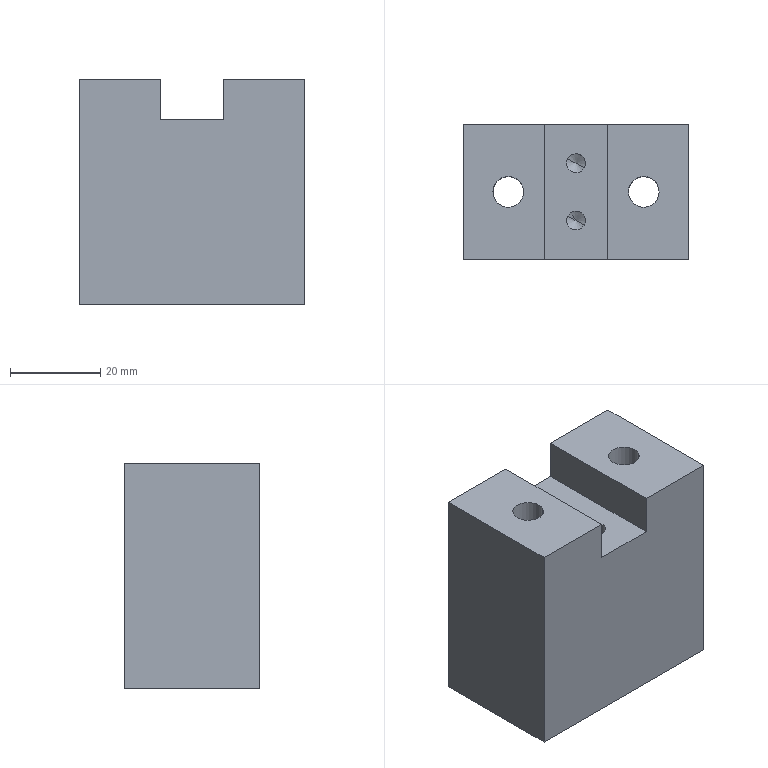Part | STEP file | 20307 | 1 solid | 26 faces | box 50 x 30 x 50 mm | volume 67161 mm3 | cylinder 12 | plane 10 | cone 4 | commonest cylinder face diameters 6.8 x8 4.2 x4
STEP:
#1=CARTESIAN_POINT('',(-17.984,-1.63,0.));
#2=VERTEX_POINT('',#1);
#3=CARTESIAN_POINT('',(-12.016,1.63,0.));
#4=VERTEX_POINT('',#3);
#5=CARTESIAN_POINT('',(-15.,0.,0.));
#6=DIRECTION('',(0.,0.,1.));
#7=AXIS2_PLACEMENT_3D('',#5,#6,$);
#8=CIRCLE('',#7,3.4);
#9=EDGE_CURVE('',#2,#4,#8,.T.);
#10=ORIENTED_EDGE('',*,*,#9,.F.);
#11=CARTESIAN_POINT('',(-17.984,-1.63,15.));
#12=VERTEX_POINT('',#11);
#13=CARTESIAN_POINT('',(-17.984,-1.63,7.345));
#14=DIRECTION('',(0.,0.,1.));
#15=VECTOR('',#14,1.);
#16=LINE('',#13,#15);
#17=EDGE_CURVE('',#12,#2,#16,.F.);
#18=ORIENTED_EDGE('',*,*,#17,.F.);
#19=CARTESIAN_POINT('',(-12.016,-1.63,15.));
#20=VERTEX_POINT('',#19);
#21=CARTESIAN_POINT('',(-15.,0.,15.));
#22=DIRECTION('',(0.,0.,1.));
#23=AXIS2_PLACEMENT_3D('',#21,#22,$);
#24=CIRCLE('',#23,3.4);
#25=EDGE_CURVE('',#20,#12,#24,.F.);
#26=ORIENTED_EDGE('',*,*,#25,.F.);
#27=CARTESIAN_POINT('',(-12.016,1.63,15.));
#28=VERTEX_POINT('',#27);
#29=CARTESIAN_POINT('',(-15.,0.,15.));
#30=DIRECTION('',(0.,0.,1.));
#31=AXIS2_PLACEMENT_3D('',#29,#30,$);
#32=CIRCLE('',#31,3.4);
#33=EDGE_CURVE('',#28,#20,#32,.F.);
#34=ORIENTED_EDGE('',*,*,#33,.F.);
#35=CARTESIAN_POINT('',(-12.016,1.63,7.345));
#36=DIRECTION('',(0.,0.,1.));
#37=VECTOR('',#36,1.);
#38=LINE('',#35,#37);
#39=EDGE_CURVE('',#28,#4,#38,.F.);
#40=ORIENTED_EDGE('',*,*,#39,.T.);
#41=EDGE_LOOP('',(#10,#18,#26,#34,#40));
#42=FACE_OUTER_BOUND('',#41,.T.);
#43=CARTESIAN_POINT('',(-15.,0.,0.1));
#44=DIRECTION('',(0.,0.,1.));
#45=DIRECTION('',(0.8776,0.4794,0.));
#46=AXIS2_PLACEMENT_3D('',#43,#44,#45);
#47=CYLINDRICAL_SURFACE('',#46,3.4);
#48=ADVANCED_FACE('',(#42),#47,.F.);
#49=CARTESIAN_POINT('',(-15.,0.,0.));
#50=DIRECTION('',(0.,0.,1.));
#51=AXIS2_PLACEMENT_3D('',#49,#50,$);
#52=CIRCLE('',#51,3.4);
#53=EDGE_CURVE('',#4,#2,#52,.T.);
#54=ORIENTED_EDGE('',*,*,#53,.F.);
#55=ORIENTED_EDGE('',*,*,#39,.F.);
#56=CARTESIAN_POINT('',(-17.984,1.63,15.));
#57=VERTEX_POINT('',#56);
#58=CARTESIAN_POINT('',(-15.,0.,15.));
#59=DIRECTION('',(0.,0.,1.));
#60=AXIS2_PLACEMENT_3D('',#58,#59,$);
#61=CIRCLE('',#60,3.4);
#62=EDGE_CURVE('',#57,#28,#61,.F.);
#63=ORIENTED_EDGE('',*,*,#62,.F.);
#64=CARTESIAN_POINT('',(-15.,0.,15.));
#65=DIRECTION('',(0.,0.,1.));
#66=AXIS2_PLACEMENT_3D('',#64,#65,$);
#67=CIRCLE('',#66,3.4);
#68=EDGE_CURVE('',#12,#57,#67,.F.);
#69=ORIENTED_EDGE('',*,*,#68,.F.);
#70=ORIENTED_EDGE('',*,*,#17,.T.);
#71=EDGE_LOOP('',(#54,#55,#63,#69,#70));
#72=FACE_OUTER_BOUND('',#71,.T.);
#73=ADVANCED_FACE('',(#72),#47,.F.);
#74=CARTESIAN_POINT('',(-7.,15.,50.));
#75=VERTEX_POINT('',#74);
#76=CARTESIAN_POINT('',(-7.,15.,41.));
#77=VERTEX_POINT('',#76);
#78=CARTESIAN_POINT('',(-7.,15.,45.5));
#79=DIRECTION('',(0.,0.,-1.));
#80=VECTOR('',#79,1.);
#81=LINE('',#78,#80);
#82=EDGE_CURVE('',#75,#77,#81,.T.);
#83=ORIENTED_EDGE('',*,*,#82,.T.);
#84=CARTESIAN_POINT('',(7.,15.,41.));
#85=VERTEX_POINT('',#84);
#86=CARTESIAN_POINT('',(0.,15.,41.));
#87=DIRECTION('',(1.,0.,0.));
#88=VECTOR('',#87,1.);
#89=LINE('',#86,#88);
#90=EDGE_CURVE('',#77,#85,#89,.T.);
#91=ORIENTED_EDGE('',*,*,#90,.T.);
#92=CARTESIAN_POINT('',(7.,15.,50.));
#93=VERTEX_POINT('',#92);
#94=CARTESIAN_POINT('',(7.,15.,45.5));
#95=DIRECTION('',(0.,0.,-1.));
#96=VECTOR('',#95,1.);
#97=LINE('',#94,#96);
#98=EDGE_CURVE('',#93,#85,#97,.T.);
#99=ORIENTED_EDGE('',*,*,#98,.F.);
#100=CARTESIAN_POINT('',(25.,15.,50.));
#101=VERTEX_POINT('',#100);
#102=CARTESIAN_POINT('',(16.,15.,50.));
#103=DIRECTION('',(1.,0.,0.));
#104=VECTOR('',#103,1.);
#105=LINE('',#102,#104);
#106=EDGE_CURVE('',#101,#93,#105,.F.);
#107=ORIENTED_EDGE('',*,*,#106,.F.);
#108=CARTESIAN_POINT('',(25.,15.,0.));
#109=VERTEX_POINT('',#108);
#110=CARTESIAN_POINT('',(25.,15.,25.));
#111=DIRECTION('',(0.,0.,1.));
#112=VECTOR('',#111,1.);
#113=LINE('',#110,#112);
#114=EDGE_CURVE('',#109,#101,#113,.T.);
#115=ORIENTED_EDGE('',*,*,#114,.F.);
#116=CARTESIAN_POINT('',(-25.,15.,0.));
#117=VERTEX_POINT('',#116);
#118=CARTESIAN_POINT('',(0.,15.,0.));
#119=DIRECTION('',(1.,0.,0.));
#120=VECTOR('',#119,1.);
#121=LINE('',#118,#120);
#122=EDGE_CURVE('',#109,#117,#121,.F.);
#123=ORIENTED_EDGE('',*,*,#122,.T.);
#124=CARTESIAN_POINT('',(-25.,15.,50.));
#125=VERTEX_POINT('',#124);
#126=CARTESIAN_POINT('',(-25.,15.,25.));
#127=DIRECTION('',(0.,0.,1.));
#128=VECTOR('',#127,1.);
#129=LINE('',#126,#128);
#130=EDGE_CURVE('',#117,#125,#129,.T.);
#131=ORIENTED_EDGE('',*,*,#130,.T.);
#132=CARTESIAN_POINT('',(-16.,15.,50.));
#133=DIRECTION('',(1.,0.,0.));
#134=VECTOR('',#133,1.);
#135=LINE('',#132,#134);
#136=EDGE_CURVE('',#75,#125,#135,.F.);
#137=ORIENTED_EDGE('',*,*,#136,.F.);
#138=EDGE_LOOP('',(#83,#91,#99,#107,#115,#123,#131,#137));
#139=FACE_OUTER_BOUND('',#138,.T.);
#140=CARTESIAN_POINT('',(-25.,15.,0.));
#141=DIRECTION('',(0.,-1.,0.));
#142=DIRECTION('',(1.,0.,0.));
#143=AXIS2_PLACEMENT_3D('',#140,#141,#142);
#144=PLANE('',#143);
#145=ADVANCED_FACE('',(#139),#144,.F.);
#146=ORIENTED_EDGE('',*,*,#130,.F.);
#147=CARTESIAN_POINT('',(-25.,-15.,0.));
#148=VERTEX_POINT('',#147);
#149=CARTESIAN_POINT('',(-25.,0.,0.));
#150=DIRECTION('',(0.,1.,0.));
#151=VECTOR('',#150,1.);
#152=LINE('',#149,#151);
#153=EDGE_CURVE('',#117,#148,#152,.F.);
#154=ORIENTED_EDGE('',*,*,#153,.T.);
#155=CARTESIAN_POINT('',(-25.,-15.,50.));
#156=VERTEX_POINT('',#155);
#157=CARTESIAN_POINT('',(-25.,-15.,25.));
#158=DIRECTION('',(0.,0.,1.));
#159=VECTOR('',#158,1.);
#160=LINE('',#157,#159);
#161=EDGE_CURVE('',#148,#156,#160,.T.);
#162=ORIENTED_EDGE('',*,*,#161,.T.);
#163=CARTESIAN_POINT('',(-25.,0.,50.));
#164=DIRECTION('',(0.,1.,0.));
#165=VECTOR('',#164,1.);
#166=LINE('',#163,#165);
#167=EDGE_CURVE('',#125,#156,#166,.F.);
#168=ORIENTED_EDGE('',*,*,#167,.F.);
#169=EDGE_LOOP('',(#146,#154,#162,#168));
#170=FACE_OUTER_BOUND('',#169,.T.);
#171=CARTESIAN_POINT('',(-25.,-15.,0.));
#172=DIRECTION('',(1.,0.,0.));
#173=DIRECTION('',(0.,1.,0.));
#174=AXIS2_PLACEMENT_3D('',#171,#172,#173);
#175=PLANE('',#174);
#176=ADVANCED_FACE('',(#170),#175,.F.);
#177=CARTESIAN_POINT('',(7.,-15.,50.));
#178=VERTEX_POINT('',#177);
#179=CARTESIAN_POINT('',(7.,-15.,41.));
#180=VERTEX_POINT('',#179);
#181=CARTESIAN_POINT('',(7.,-15.,45.5));
#182=DIRECTION('',(0.,0.,-1.));
#183=VECTOR('',#182,1.);
#184=LINE('',#181,#183);
#185=EDGE_CURVE('',#178,#180,#184,.T.);
#186=ORIENTED_EDGE('',*,*,#185,.T.);
#187=CARTESIAN_POINT('',(-7.,-15.,41.));
#188=VERTEX_POINT('',#187);
#189=CARTESIAN_POINT('',(0.,-15.,41.));
#190=DIRECTION('',(1.,0.,0.));
#191=VECTOR('',#190,1.);
#192=LINE('',#189,#191);
#193=EDGE_CURVE('',#188,#180,#192,.T.);
#194=ORIENTED_EDGE('',*,*,#193,.F.);
#195=CARTESIAN_POINT('',(-7.,-15.,50.));
#196=VERTEX_POINT('',#195);
#197=CARTESIAN_POINT('',(-7.,-15.,45.5));
#198=DIRECTION('',(0.,0.,-1.));
#199=VECTOR('',#198,1.);
#200=LINE('',#197,#199);
#201=EDGE_CURVE('',#196,#188,#200,.T.);
#202=ORIENTED_EDGE('',*,*,#201,.F.);
#203=CARTESIAN_POINT('',(-16.,-15.,50.));
#204=DIRECTION('',(-1.,0.,0.));
#205=VECTOR('',#204,1.);
#206=LINE('',#203,#205);
#207=EDGE_CURVE('',#156,#196,#206,.F.);
#208=ORIENTED_EDGE('',*,*,#207,.F.);
#209=ORIENTED_EDGE('',*,*,#161,.F.);
#210=CARTESIAN_POINT('',(25.,-15.,0.));
#211=VERTEX_POINT('',#210);
#212=CARTESIAN_POINT('',(0.,-15.,0.));
#213=DIRECTION('',(-1.,0.,0.));
#214=VECTOR('',#213,1.);
#215=LINE('',#212,#214);
#216=EDGE_CURVE('',#148,#211,#215,.F.);
#217=ORIENTED_EDGE('',*,*,#216,.T.);
#218=CARTESIAN_POINT('',(25.,-15.,50.));
#219=VERTEX_POINT('',#218);
#220=CARTESIAN_POINT('',(25.,-15.,25.));
#221=DIRECTION('',(0.,0.,1.));
#222=VECTOR('',#221,1.);
#223=LINE('',#220,#222);
#224=EDGE_CURVE('',#211,#219,#223,.T.);
#225=ORIENTED_EDGE('',*,*,#224,.T.);
#226=CARTESIAN_POINT('',(16.,-15.,50.));
#227=DIRECTION('',(-1.,0.,0.));
#228=VECTOR('',#227,1.);
#229=LINE('',#226,#228);
#230=EDGE_CURVE('',#178,#219,#229,.F.);
#231=ORIENTED_EDGE('',*,*,#230,.F.);
#232=EDGE_LOOP('',(#186,#194,#202,#208,#209,#217,#225,#231));
#233=FACE_OUTER_BOUND('',#232,.T.);
#234=CARTESIAN_POINT('',(25.,-15.,0.));
#235=DIRECTION('',(0.,1.,0.));
#236=DIRECTION('',(-1.,0.,0.));
#237=AXIS2_PLACEMENT_3D('',#234,#235,#236);
#238=PLANE('',#237);
#239=ADVANCED_FACE('',(#233),#238,.F.);
#240=ORIENTED_EDGE('',*,*,#193,.T.);
#241=CARTESIAN_POINT('',(7.,0.,41.));
#242=DIRECTION('',(0.,-1.,0.));
#243=VECTOR('',#242,1.);
#244=LINE('',#241,#243);
#245=EDGE_CURVE('',#180,#85,#244,.F.);
#246=ORIENTED_EDGE('',*,*,#245,.T.);
#247=ORIENTED_EDGE('',*,*,#90,.F.);
#248=CARTESIAN_POINT('',(-7.,0.,41.));
#249=DIRECTION('',(0.,1.,0.));
#250=VECTOR('',#249,1.);
#251=LINE('',#248,#250);
#252=EDGE_CURVE('',#77,#188,#251,.F.);
#253=ORIENTED_EDGE('',*,*,#252,.T.);
#254=EDGE_LOOP('',(#240,#246,#247,#253));
#255=FACE_OUTER_BOUND('',#254,.T.);
#256=CARTESIAN_POINT('',(1.843,-7.357,41.));
#257=VERTEX_POINT('',#256);
#258=CARTESIAN_POINT('',(-1.843,-5.343,41.));
#259=VERTEX_POINT('',#258);
#260=CARTESIAN_POINT('',(0.,-6.35,41.));
#261=DIRECTION('',(0.,0.,1.));
#262=AXIS2_PLACEMENT_3D('',#260,#261,$);
#263=CIRCLE('',#262,2.1);
#264=EDGE_CURVE('',#257,#259,#263,.T.);
#265=ORIENTED_EDGE('',*,*,#264,.F.);
#266=CARTESIAN_POINT('',(0.,-6.35,41.));
#267=DIRECTION('',(0.,0.,1.));
#268=AXIS2_PLACEMENT_3D('',#266,#267,$);
#269=CIRCLE('',#268,2.1);
#270=EDGE_CURVE('',#259,#257,#269,.T.);
#271=ORIENTED_EDGE('',*,*,#270,.F.);
#272=EDGE_LOOP('',(#265,#271));
#273=FACE_BOUND('',#272,.T.);
#274=CARTESIAN_POINT('',(-1.843,7.357,41.));
#275=VERTEX_POINT('',#274);
#276=CARTESIAN_POINT('',(1.843,5.343,41.));
#277=VERTEX_POINT('',#276);
#278=CARTESIAN_POINT('',(0.,6.35,41.));
#279=DIRECTION('',(0.,0.,1.));
#280=AXIS2_PLACEMENT_3D('',#278,#279,$);
#281=CIRCLE('',#280,2.1);
#282=EDGE_CURVE('',#275,#277,#281,.T.);
#283=ORIENTED_EDGE('',*,*,#282,.F.);
#284=CARTESIAN_POINT('',(0.,6.35,41.));
#285=DIRECTION('',(0.,0.,1.));
#286=AXIS2_PLACEMENT_3D('',#284,#285,$);
#287=CIRCLE('',#286,2.1);
#288=EDGE_CURVE('',#277,#275,#287,.T.);
#289=ORIENTED_EDGE('',*,*,#288,.F.);
#290=EDGE_LOOP('',(#283,#289));
#291=FACE_BOUND('',#290,.T.);
#292=CARTESIAN_POINT('',(0.,0.,41.));
#293=DIRECTION('',(0.,0.,1.));
#294=DIRECTION('',(1.,0.,0.));
#295=AXIS2_PLACEMENT_3D('',#292,#293,#294);
#296=PLANE('',#295);
#297=ADVANCED_FACE('',(#255,#273,#291),#296,.T.);
#298=CARTESIAN_POINT('',(12.016,-1.63,0.));
#299=VERTEX_POINT('',#298);
#300=CARTESIAN_POINT('',(17.984,1.63,0.));
#301=VERTEX_POINT('',#300);
#302=CARTESIAN_POINT('',(15.,0.,0.));
#303=DIRECTION('',(0.,0.,1.));
#304=AXIS2_PLACEMENT_3D('',#302,#303,$);
#305=CIRCLE('',#304,3.4);
#306=EDGE_CURVE('',#299,#301,#305,.T.);
#307=ORIENTED_EDGE('',*,*,#306,.F.);
#308=CARTESIAN_POINT('',(12.016,-1.63,15.));
#309=VERTEX_POINT('',#308);
#310=CARTESIAN_POINT('',(12.016,-1.63,7.345));
#311=DIRECTION('',(0.,0.,1.));
#312=VECTOR('',#311,1.);
#313=LINE('',#310,#312);
#314=EDGE_CURVE('',#309,#299,#313,.F.);
#315=ORIENTED_EDGE('',*,*,#314,.F.);
#316=CARTESIAN_POINT('',(17.984,-1.63,15.));
#317=VERTEX_POINT('',#316);
#318=CARTESIAN_POINT('',(15.,0.,15.));
#319=DIRECTION('',(0.,0.,1.));
#320=AXIS2_PLACEMENT_3D('',#318,#319,$);
#321=CIRCLE('',#320,3.4);
#322=EDGE_CURVE('',#317,#309,#321,.F.);
#323=ORIENTED_EDGE('',*,*,#322,.F.);
#324=CARTESIAN_POINT('',(17.984,1.63,15.));
#325=VERTEX_POINT('',#324);
#326=CARTESIAN_POINT('',(15.,0.,15.));
#327=DIRECTION('',(0.,0.,1.));
#328=AXIS2_PLACEMENT_3D('',#326,#327,$);
#329=CIRCLE('',#328,3.4);
#330=EDGE_CURVE('',#325,#317,#329,.F.);
#331=ORIENTED_EDGE('',*,*,#330,.F.);
#332=CARTESIAN_POINT('',(17.984,1.63,7.345));
#333=DIRECTION('',(0.,0.,1.));
#334=VECTOR('',#333,1.);
#335=LINE('',#332,#334);
#336=EDGE_CURVE('',#325,#301,#335,.F.);
#337=ORIENTED_EDGE('',*,*,#336,.T.);
#338=EDGE_LOOP('',(#307,#315,#323,#331,#337));
#339=FACE_OUTER_BOUND('',#338,.T.);
#340=CARTESIAN_POINT('',(15.,0.,0.1));
#341=DIRECTION('',(0.,0.,1.));
#342=DIRECTION('',(0.8776,0.4794,0.));
#343=AXIS2_PLACEMENT_3D('',#340,#341,#342);
#344=CYLINDRICAL_SURFACE('',#343,3.4);
#345=ADVANCED_FACE('',(#339),#344,.F.);
#346=CARTESIAN_POINT('',(15.,0.,0.));
#347=DIRECTION('',(0.,0.,1.));
#348=AXIS2_PLACEMENT_3D('',#346,#347,$);
#349=CIRCLE('',#348,3.4);
#350=EDGE_CURVE('',#301,#299,#349,.T.);
#351=ORIENTED_EDGE('',*,*,#350,.F.);
#352=ORIENTED_EDGE('',*,*,#336,.F.);
#353=CARTESIAN_POINT('',(12.016,1.63,15.));
#354=VERTEX_POINT('',#353);
#355=CARTESIAN_POINT('',(15.,0.,15.));
#356=DIRECTION('',(0.,0.,1.));
#357=AXIS2_PLACEMENT_3D('',#355,#356,$);
#358=CIRCLE('',#357,3.4);
#359=EDGE_CURVE('',#354,#325,#358,.F.);
#360=ORIENTED_EDGE('',*,*,#359,.F.);
#361=CARTESIAN_POINT('',(15.,0.,15.));
#362=DIRECTION('',(0.,0.,1.));
#363=AXIS2_PLACEMENT_3D('',#361,#362,$);
#364=CIRCLE('',#363,3.4);
#365=EDGE_CURVE('',#309,#354,#364,.F.);
#366=ORIENTED_EDGE('',*,*,#365,.F.);
#367=ORIENTED_EDGE('',*,*,#314,.T.);
#368=EDGE_LOOP('',(#351,#352,#360,#366,#367));
#369=FACE_OUTER_BOUND('',#368,.T.);
#370=ADVANCED_FACE('',(#369),#344,.F.);
#371=CARTESIAN_POINT('',(0.,-6.35,24.788));
#372=VERTEX_POINT('',#371);
#373=CARTESIAN_POINT('',(1.843,-7.357,26.));
#374=VERTEX_POINT('',#373);
#375=CARTESIAN_POINT('',(0.9215,-6.853,25.394));
#376=DIRECTION('',(0.76,-0.4152,0.5));
#377=VECTOR('',#376,1.);
#378=LINE('',#375,#377);
#379=EDGE_CURVE('',#372,#374,#378,.T.);
#380=ORIENTED_EDGE('',*,*,#379,.T.);
#381=CARTESIAN_POINT('',(-1.843,-5.343,26.));
#382=VERTEX_POINT('',#381);
#383=CARTESIAN_POINT('',(0.,-6.35,26.));
#384=DIRECTION('',(0.,0.,1.));
#385=AXIS2_PLACEMENT_3D('',#383,#384,$);
#386=CIRCLE('',#385,2.1);
#387=EDGE_CURVE('',#382,#374,#386,.F.);
#388=ORIENTED_EDGE('',*,*,#387,.F.);
#389=CARTESIAN_POINT('',(-0.9215,-5.847,25.394));
#390=DIRECTION('',(-0.76,0.4152,0.5));
#391=VECTOR('',#390,1.);
#392=LINE('',#389,#391);
#393=EDGE_CURVE('',#372,#382,#392,.T.);
#394=ORIENTED_EDGE('',*,*,#393,.F.);
#395=EDGE_LOOP('',(#380,#388,#394));
#396=FACE_OUTER_BOUND('',#395,.T.);
#397=CARTESIAN_POINT('',(0.,-6.35,24.788));
#398=DIRECTION('',(0.,0.,1.));
#399=DIRECTION('',(0.8776,-0.4794,0.));
#400=AXIS2_PLACEMENT_3D('',#397,#398,#399);
#401=CONICAL_SURFACE('',#400,0.,1.047);
#402=ADVANCED_FACE('',(#396),#401,.F.);
#403=CARTESIAN_POINT('',(0.,6.35,24.788));
#404=VERTEX_POINT('',#403);
#405=CARTESIAN_POINT('',(-1.843,7.357,26.));
#406=VERTEX_POINT('',#405);
#407=CARTESIAN_POINT('',(-0.9215,6.853,25.394));
#408=DIRECTION('',(-0.76,0.4152,0.5));
#409=VECTOR('',#408,1.);
#410=LINE('',#407,#409);
#411=EDGE_CURVE('',#404,#406,#410,.T.);
#412=ORIENTED_EDGE('',*,*,#411,.T.);
#413=CARTESIAN_POINT('',(1.843,5.343,26.));
#414=VERTEX_POINT('',#413);
#415=CARTESIAN_POINT('',(0.,6.35,26.));
#416=DIRECTION('',(0.,0.,1.));
#417=AXIS2_PLACEMENT_3D('',#415,#416,$);
#418=CIRCLE('',#417,2.1);
#419=EDGE_CURVE('',#414,#406,#418,.F.);
#420=ORIENTED_EDGE('',*,*,#419,.F.);
#421=CARTESIAN_POINT('',(0.9215,5.847,25.394));
#422=DIRECTION('',(0.76,-0.4152,0.5));
#423=VECTOR('',#422,1.);
#424=LINE('',#421,#423);
#425=EDGE_CURVE('',#404,#414,#424,.T.);
#426=ORIENTED_EDGE('',*,*,#425,.F.);
#427=EDGE_LOOP('',(#412,#420,#426));
#428=FACE_OUTER_BOUND('',#427,.T.);
#429=CARTESIAN_POINT('',(0.,6.35,24.788));
#430=DIRECTION('',(0.,0.,1.));
#431=DIRECTION('',(0.8776,-0.4794,0.));
#432=AXIS2_PLACEMENT_3D('',#429,#430,#431);
#433=CONICAL_SURFACE('',#432,0.,1.047);
#434=ADVANCED_FACE('',(#428),#433,.F.);
#435=ORIENTED_EDGE('',*,*,#425,.T.);
#436=CARTESIAN_POINT('',(0.,6.35,26.));
#437=DIRECTION('',(0.,0.,1.));
#438=AXIS2_PLACEMENT_3D('',#436,#437,$);
#439=CIRCLE('',#438,2.1);
#440=EDGE_CURVE('',#406,#414,#439,.F.);
#441=ORIENTED_EDGE('',*,*,#440,.F.);
#442=ORIENTED_EDGE('',*,*,#411,.F.);
#443=EDGE_LOOP('',(#435,#441,#442));
#444=FACE_OUTER_BOUND('',#443,.T.);
#445=ADVANCED_FACE('',(#444),#433,.F.);
#446=ORIENTED_EDGE('',*,*,#393,.T.);
#447=CARTESIAN_POINT('',(0.,-6.35,26.));
#448=DIRECTION('',(0.,0.,1.));
#449=AXIS2_PLACEMENT_3D('',#447,#448,$);
#450=CIRCLE('',#449,2.1);
#451=EDGE_CURVE('',#374,#382,#450,.F.);
#452=ORIENTED_EDGE('',*,*,#451,.F.);
#453=ORIENTED_EDGE('',*,*,#379,.F.);
#454=EDGE_LOOP('',(#446,#452,#453));
#455=FACE_OUTER_BOUND('',#454,.T.);
#456=ADVANCED_FACE('',(#455),#401,.F.);
#457=ORIENTED_EDGE('',*,*,#288,.T.);
#458=CARTESIAN_POINT('',(-1.843,7.357,38.155));
#459=DIRECTION('',(0.,0.,-1.));
#460=VECTOR('',#459,1.);
#461=LINE('',#458,#460);
#462=EDGE_CURVE('',#406,#275,#461,.F.);
#463=ORIENTED_EDGE('',*,*,#462,.F.);
#464=ORIENTED_EDGE('',*,*,#440,.T.);
#465=CARTESIAN_POINT('',(1.843,5.343,38.155));
#466=DIRECTION('',(0.,0.,-1.));
#467=VECTOR('',#466,1.);
#468=LINE('',#465,#467);
#469=EDGE_CURVE('',#414,#277,#468,.F.);
#470=ORIENTED_EDGE('',*,*,#469,.T.);
#471=EDGE_LOOP('',(#457,#463,#464,#470));
#472=FACE_OUTER_BOUND('',#471,.T.);
#473=CARTESIAN_POINT('',(0.,6.35,40.9));
#474=DIRECTION('',(0.,0.,-1.));
#475=DIRECTION('',(0.8776,-0.4794,0.));
#476=AXIS2_PLACEMENT_3D('',#473,#474,#475);
#477=CYLINDRICAL_SURFACE('',#476,2.1);
#478=ADVANCED_FACE('',(#472),#477,.F.);
#479=ORIENTED_EDGE('',*,*,#282,.T.);
#480=ORIENTED_EDGE('',*,*,#469,.F.);
#481=ORIENTED_EDGE('',*,*,#419,.T.);
#482=ORIENTED_EDGE('',*,*,#462,.T.);
#483=EDGE_LOOP('',(#479,#480,#481,#482));
#484=FACE_OUTER_BOUND('',#483,.T.);
#485=ADVANCED_FACE('',(#484),#477,.F.);
#486=ORIENTED_EDGE('',*,*,#270,.T.);
#487=CARTESIAN_POINT('',(1.843,-7.357,38.155));
#488=DIRECTION('',(0.,0.,-1.));
#489=VECTOR('',#488,1.);
#490=LINE('',#487,#489);
#491=EDGE_CURVE('',#374,#257,#490,.F.);
#492=ORIENTED_EDGE('',*,*,#491,.F.);
#493=ORIENTED_EDGE('',*,*,#451,.T.);
#494=CARTESIAN_POINT('',(-1.843,-5.343,38.155));
#495=DIRECTION('',(0.,0.,-1.));
#496=VECTOR('',#495,1.);
#497=LINE('',#494,#496);
#498=EDGE_CURVE('',#382,#259,#497,.F.);
#499=ORIENTED_EDGE('',*,*,#498,.T.);
#500=EDGE_LOOP('',(#486,#492,#493,#499));
#501=FACE_OUTER_BOUND('',#500,.T.);
#502=CARTESIAN_POINT('',(0.,-6.35,40.9));
#503=DIRECTION('',(0.,0.,-1.));
#504=DIRECTION('',(0.8776,-0.4794,0.));
#505=AXIS2_PLACEMENT_3D('',#502,#503,#504);
#506=CYLINDRICAL_SURFACE('',#505,2.1);
#507=ADVANCED_FACE('',(#501),#506,.F.);
#508=ORIENTED_EDGE('',*,*,#264,.T.);
#509=ORIENTED_EDGE('',*,*,#498,.F.);
#510=ORIENTED_EDGE('',*,*,#387,.T.);
#511=ORIENTED_EDGE('',*,*,#491,.T.);
#512=EDGE_LOOP('',(#508,#509,#510,#511));
#513=FACE_OUTER_BOUND('',#512,.T.);
#514=ADVANCED_FACE('',(#513),#506,.F.);
#515=ORIENTED_EDGE('',*,*,#245,.F.);
#516=ORIENTED_EDGE('',*,*,#185,.F.);
#517=CARTESIAN_POINT('',(7.,0.,50.));
#518=DIRECTION('',(0.,-1.,0.));
#519=VECTOR('',#518,1.);
#520=LINE('',#517,#519);
#521=EDGE_CURVE('',#178,#93,#520,.F.);
#522=ORIENTED_EDGE('',*,*,#521,.T.);
#523=ORIENTED_EDGE('',*,*,#98,.T.);
#524=EDGE_LOOP('',(#515,#516,#522,#523));
#525=FACE_OUTER_BOUND('',#524,.T.);
#526=CARTESIAN_POINT('',(7.,25.,50.));
#527=DIRECTION('',(1.,0.,0.));
#528=DIRECTION('',(0.,-1.,0.));
#529=AXIS2_PLACEMENT_3D('',#526,#527,#528);
#530=PLANE('',#529);
#531=ADVANCED_FACE('',(#525),#530,.F.);
#532=ORIENTED_EDGE('',*,*,#224,.F.);
#533=CARTESIAN_POINT('',(25.,0.,0.));
#534=DIRECTION('',(0.,-1.,0.));
#535=VECTOR('',#534,1.);
#536=LINE('',#533,#535);
#537=EDGE_CURVE('',#211,#109,#536,.F.);
#538=ORIENTED_EDGE('',*,*,#537,.T.);
#539=ORIENTED_EDGE('',*,*,#114,.T.);
#540=CARTESIAN_POINT('',(25.,0.,50.));
#541=DIRECTION('',(0.,-1.,0.));
#542=VECTOR('',#541,1.);
#543=LINE('',#540,#542);
#544=EDGE_CURVE('',#219,#101,#543,.F.);
#545=ORIENTED_EDGE('',*,*,#544,.F.);
#546=EDGE_LOOP('',(#532,#538,#539,#545));
#547=FACE_OUTER_BOUND('',#546,.T.);
#548=CARTESIAN_POINT('',(25.,15.,0.));
#549=DIRECTION('',(-1.,0.,0.));
#550=DIRECTION('',(0.,-1.,0.));
#551=AXIS2_PLACEMENT_3D('',#548,#549,#550);
#552=PLANE('',#551);
#553=ADVANCED_FACE('',(#547),#552,.F.);
#554=ORIENTED_EDGE('',*,*,#252,.F.);
#555=ORIENTED_EDGE('',*,*,#82,.F.);
#556=CARTESIAN_POINT('',(-7.,0.,50.));
#557=DIRECTION('',(0.,1.,0.));
#558=VECTOR('',#557,1.);
#559=LINE('',#556,#558);
#560=EDGE_CURVE('',#75,#196,#559,.F.);
#561=ORIENTED_EDGE('',*,*,#560,.T.);
#562=ORIENTED_EDGE('',*,*,#201,.T.);
#563=EDGE_LOOP('',(#554,#555,#561,#562));
#564=FACE_OUTER_BOUND('',#563,.T.);
#565=CARTESIAN_POINT('',(-7.,-25.,50.));
#566=DIRECTION('',(-1.,0.,0.));
#567=DIRECTION('',(0.,1.,0.));
#568=AXIS2_PLACEMENT_3D('',#565,#566,#567);
#569=PLANE('',#568);
#570=ADVANCED_FACE('',(#564),#569,.F.);
#571=ORIENTED_EDGE('',*,*,#537,.F.);
#572=ORIENTED_EDGE('',*,*,#216,.F.);
#573=ORIENTED_EDGE('',*,*,#153,.F.);
#574=ORIENTED_EDGE('',*,*,#122,.F.);
#575=EDGE_LOOP('',(#571,#572,#573,#574));
#576=FACE_OUTER_BOUND('',#575,.T.);
#577=ORIENTED_EDGE('',*,*,#350,.T.);
#578=ORIENTED_EDGE('',*,*,#306,.T.);
#579=EDGE_LOOP('',(#577,#578));
#580=FACE_BOUND('',#579,.T.);
#581=ORIENTED_EDGE('',*,*,#9,.T.);
#582=ORIENTED_EDGE('',*,*,#53,.T.);
#583=EDGE_LOOP('',(#581,#582));
#584=FACE_BOUND('',#583,.T.);
#585=CARTESIAN_POINT('',(0.,0.,0.));
#586=DIRECTION('',(0.,0.,1.));
#587=DIRECTION('',(1.,0.,0.));
#588=AXIS2_PLACEMENT_3D('',#585,#586,#587);
#589=PLANE('',#588);
#590=ADVANCED_FACE('',(#576,#580,#584),#589,.F.);
#591=CARTESIAN_POINT('',(-12.016,-1.63,50.));
#592=VERTEX_POINT('',#591);
#593=CARTESIAN_POINT('',(-17.984,1.63,50.));
#594=VERTEX_POINT('',#593);
#595=CARTESIAN_POINT('',(-15.,0.,50.));
#596=DIRECTION('',(0.,0.,-1.));
#597=AXIS2_PLACEMENT_3D('',#595,#596,$);
#598=CIRCLE('',#597,3.4);
#599=EDGE_CURVE('',#592,#594,#598,.F.);
#600=ORIENTED_EDGE('',*,*,#599,.T.);
#601=CARTESIAN_POINT('',(-17.984,1.63,32.655));
#602=DIRECTION('',(0.,0.,-1.));
#603=VECTOR('',#602,1.);
#604=LINE('',#601,#603);
#605=EDGE_CURVE('',#57,#594,#604,.F.);
#606=ORIENTED_EDGE('',*,*,#605,.F.);
#607=ORIENTED_EDGE('',*,*,#62,.T.);
#608=ORIENTED_EDGE('',*,*,#33,.T.);
#609=CARTESIAN_POINT('',(-12.016,-1.63,32.655));
#610=DIRECTION('',(0.,0.,-1.));
#611=VECTOR('',#610,1.);
#612=LINE('',#609,#611);
#613=EDGE_CURVE('',#20,#592,#612,.F.);
#614=ORIENTED_EDGE('',*,*,#613,.T.);
#615=EDGE_LOOP('',(#600,#606,#607,#608,#614));
#616=FACE_OUTER_BOUND('',#615,.T.);
#617=CARTESIAN_POINT('',(-15.,0.,49.9));
#618=DIRECTION('',(0.,0.,-1.));
#619=DIRECTION('',(0.8776,-0.4794,0.));
#620=AXIS2_PLACEMENT_3D('',#617,#618,#619);
#621=CYLINDRICAL_SURFACE('',#620,3.4);
#622=ADVANCED_FACE('',(#616),#621,.F.);
#623=CARTESIAN_POINT('',(-15.,0.,50.));
#624=DIRECTION('',(0.,0.,-1.));
#625=AXIS2_PLACEMENT_3D('',#623,#624,$);
#626=CIRCLE('',#625,3.4);
#627=EDGE_CURVE('',#594,#592,#626,.F.);
#628=ORIENTED_EDGE('',*,*,#627,.T.);
#629=ORIENTED_EDGE('',*,*,#613,.F.);
#630=ORIENTED_EDGE('',*,*,#25,.T.);
#631=ORIENTED_EDGE('',*,*,#68,.T.);
#632=ORIENTED_EDGE('',*,*,#605,.T.);
#633=EDGE_LOOP('',(#628,#629,#630,#631,#632));
#634=FACE_OUTER_BOUND('',#633,.T.);
#635=ADVANCED_FACE('',(#634),#621,.F.);
#636=ORIENTED_EDGE('',*,*,#136,.T.);
#637=ORIENTED_EDGE('',*,*,#167,.T.);
#638=ORIENTED_EDGE('',*,*,#207,.T.);
#639=ORIENTED_EDGE('',*,*,#560,.F.);
#640=EDGE_LOOP('',(#636,#637,#638,#639));
#641=FACE_OUTER_BOUND('',#640,.T.);
#642=ORIENTED_EDGE('',*,*,#627,.F.);
#643=ORIENTED_EDGE('',*,*,#599,.F.);
#644=EDGE_LOOP('',(#642,#643));
#645=FACE_BOUND('',#644,.T.);
#646=CARTESIAN_POINT('',(0.,0.,50.));
#647=DIRECTION('',(0.,0.,1.));
#648=DIRECTION('',(1.,0.,0.));
#649=AXIS2_PLACEMENT_3D('',#646,#647,#648);
#650=PLANE('',#649);
#651=ADVANCED_FACE('',(#641,#645),#650,.T.);
#652=CARTESIAN_POINT('',(17.984,-1.63,50.));
#653=VERTEX_POINT('',#652);
#654=CARTESIAN_POINT('',(12.016,1.63,50.));
#655=VERTEX_POINT('',#654);
#656=CARTESIAN_POINT('',(15.,0.,50.));
#657=DIRECTION('',(0.,0.,-1.));
#658=AXIS2_PLACEMENT_3D('',#656,#657,$);
#659=CIRCLE('',#658,3.4);
#660=EDGE_CURVE('',#653,#655,#659,.F.);
#661=ORIENTED_EDGE('',*,*,#660,.T.);
#662=CARTESIAN_POINT('',(12.016,1.63,42.655));
#663=DIRECTION('',(0.,0.,-1.));
#664=VECTOR('',#663,1.);
#665=LINE('',#662,#664);
#666=EDGE_CURVE('',#354,#655,#665,.F.);
#667=ORIENTED_EDGE('',*,*,#666,.F.);
#668=ORIENTED_EDGE('',*,*,#359,.T.);
#669=ORIENTED_EDGE('',*,*,#330,.T.);
#670=CARTESIAN_POINT('',(17.984,-1.63,42.655));
#671=DIRECTION('',(0.,0.,-1.));
#672=VECTOR('',#671,1.);
#673=LINE('',#670,#672);
#674=EDGE_CURVE('',#317,#653,#673,.F.);
#675=ORIENTED_EDGE('',*,*,#674,.T.);
#676=EDGE_LOOP('',(#661,#667,#668,#669,#675));
#677=FACE_OUTER_BOUND('',#676,.T.);
#678=CARTESIAN_POINT('',(15.,0.,49.9));
#679=DIRECTION('',(0.,0.,-1.));
#680=DIRECTION('',(0.8776,-0.4794,0.));
#681=AXIS2_PLACEMENT_3D('',#678,#679,#680);
#682=CYLINDRICAL_SURFACE('',#681,3.4);
#683=ADVANCED_FACE('',(#677),#682,.F.);
#684=CARTESIAN_POINT('',(15.,0.,50.));
#685=DIRECTION('',(0.,0.,-1.));
#686=AXIS2_PLACEMENT_3D('',#684,#685,$);
#687=CIRCLE('',#686,3.4);
#688=EDGE_CURVE('',#655,#653,#687,.F.);
#689=ORIENTED_EDGE('',*,*,#688,.T.);
#690=ORIENTED_EDGE('',*,*,#674,.F.);
#691=ORIENTED_EDGE('',*,*,#322,.T.);
#692=ORIENTED_EDGE('',*,*,#365,.T.);
#693=ORIENTED_EDGE('',*,*,#666,.T.);
#694=EDGE_LOOP('',(#689,#690,#691,#692,#693));
#695=FACE_OUTER_BOUND('',#694,.T.);
#696=ADVANCED_FACE('',(#695),#682,.F.);
#697=ORIENTED_EDGE('',*,*,#230,.T.);
#698=ORIENTED_EDGE('',*,*,#544,.T.);
#699=ORIENTED_EDGE('',*,*,#106,.T.);
#700=ORIENTED_EDGE('',*,*,#521,.F.);
#701=EDGE_LOOP('',(#697,#698,#699,#700));
#702=FACE_OUTER_BOUND('',#701,.T.);
#703=ORIENTED_EDGE('',*,*,#660,.F.);
#704=ORIENTED_EDGE('',*,*,#688,.F.);
#705=EDGE_LOOP('',(#703,#704));
#706=FACE_BOUND('',#705,.T.);
#707=ADVANCED_FACE('',(#702,#706),#650,.T.);
#708=CLOSED_SHELL('',(#48,#73,#145,#176,#239,#297,#345,#370,#402,#434,#445,#456,#478,#485,#507,#514,#531,#553,#570,#590,#622,#635,#651,#683,#696,#707));
#709=MANIFOLD_SOLID_BREP('',#708);
#710=(LENGTH_UNIT()NAMED_UNIT(*)SI_UNIT(.MILLI.,.METRE.));
#711=UNCERTAINTY_MEASURE_WITH_UNIT(LENGTH_MEASURE(0.005),#710,'','');
#712=(NAMED_UNIT(*)PLANE_ANGLE_UNIT()SI_UNIT($,.RADIAN.));
#713=(NAMED_UNIT(*)SI_UNIT($,.STERADIAN.)SOLID_ANGLE_UNIT());
#714=(GEOMETRIC_REPRESENTATION_CONTEXT(3)GLOBAL_UNCERTAINTY_ASSIGNED_CONTEXT((#711))GLOBAL_UNIT_ASSIGNED_CONTEXT((#710,#712,#713))REPRESENTATION_CONTEXT('',''));
#715=ADVANCED_BREP_SHAPE_REPRESENTATION('',(#709),#714);